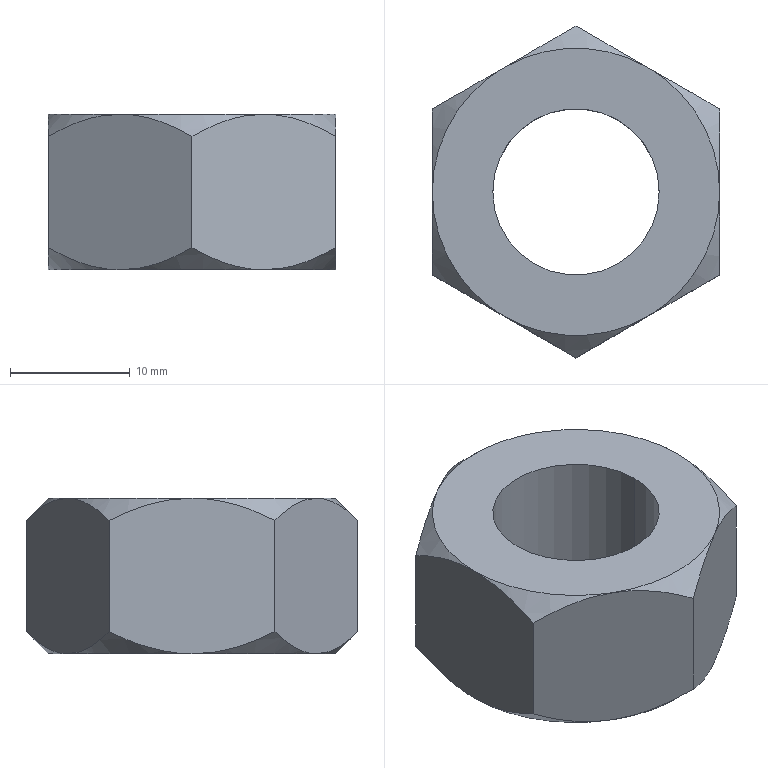Part | NX | 1 solid | 22 faces | box 24 x 27.713 x 13 mm | volume 4460 mm3 | cone 12 | plane 8 | cylinder 2 | commonest cylinder face diameters 13.9 x2
STEP:
#1=CARTESIAN_POINT('',(6.,-10.392,-6.5));
#2=VERTEX_POINT('',#1);
#3=CARTESIAN_POINT('',(12.,0.,-6.5));
#4=VERTEX_POINT('',#3);
#5=CARTESIAN_POINT('',(0.,0.,-6.5));
#6=DIRECTION('',(0.,0.,1.));
#7=DIRECTION('',(0.5,-0.866,0.));
#8=AXIS2_PLACEMENT_3D('',#5,#6,#7);
#9=CIRCLE('',#8,12.);
#10=EDGE_CURVE('',#2,#4,#9,.T.);
#11=ORIENTED_EDGE('',*,*,#10,.F.);
#12=CARTESIAN_POINT('',(-6.,-10.392,-6.5));
#13=VERTEX_POINT('',#12);
#14=CARTESIAN_POINT('',(0.,0.,-6.5));
#15=DIRECTION('',(0.,0.,1.));
#16=DIRECTION('',(-0.5,-0.866,0.));
#17=AXIS2_PLACEMENT_3D('',#14,#15,#16);
#18=CIRCLE('',#17,12.);
#19=EDGE_CURVE('',#13,#2,#18,.T.);
#20=ORIENTED_EDGE('',*,*,#19,.F.);
#21=CARTESIAN_POINT('',(-12.,0.,-6.5));
#22=VERTEX_POINT('',#21);
#23=CARTESIAN_POINT('',(0.,0.,-6.5));
#24=DIRECTION('',(0.,0.,1.));
#25=DIRECTION('',(-1.,0.,0.));
#26=AXIS2_PLACEMENT_3D('',#23,#24,#25);
#27=CIRCLE('',#26,12.);
#28=EDGE_CURVE('',#22,#13,#27,.T.);
#29=ORIENTED_EDGE('',*,*,#28,.F.);
#30=CARTESIAN_POINT('',(-6.,10.392,-6.5));
#31=VERTEX_POINT('',#30);
#32=CARTESIAN_POINT('',(0.,0.,-6.5));
#33=DIRECTION('',(0.,0.,1.));
#34=DIRECTION('',(-0.5,0.866,0.));
#35=AXIS2_PLACEMENT_3D('',#32,#33,#34);
#36=CIRCLE('',#35,12.);
#37=EDGE_CURVE('',#31,#22,#36,.T.);
#38=ORIENTED_EDGE('',*,*,#37,.F.);
#39=CARTESIAN_POINT('',(6.,10.392,-6.5));
#40=VERTEX_POINT('',#39);
#41=CARTESIAN_POINT('',(0.,0.,-6.5));
#42=DIRECTION('',(0.,0.,1.));
#43=DIRECTION('',(0.5,0.866,0.));
#44=AXIS2_PLACEMENT_3D('',#41,#42,#43);
#45=CIRCLE('',#44,12.);
#46=EDGE_CURVE('',#40,#31,#45,.T.);
#47=ORIENTED_EDGE('',*,*,#46,.F.);
#48=CARTESIAN_POINT('',(0.,0.,-6.5));
#49=DIRECTION('',(0.,0.,1.));
#50=DIRECTION('',(1.,0.,0.));
#51=AXIS2_PLACEMENT_3D('',#48,#49,#50);
#52=CIRCLE('',#51,12.);
#53=EDGE_CURVE('',#4,#40,#52,.T.);
#54=ORIENTED_EDGE('',*,*,#53,.F.);
#55=EDGE_LOOP('',(#11,#20,#29,#38,#47,#54));
#56=FACE_BOUND('',#55,.T.);
#57=CARTESIAN_POINT('',(-6.95,0.,-6.5));
#58=VERTEX_POINT('',#57);
#59=CARTESIAN_POINT('',(6.95,0.,-6.5));
#60=VERTEX_POINT('',#59);
#61=CARTESIAN_POINT('',(0.,0.,-6.5));
#62=DIRECTION('',(0.,0.,-1.));
#63=DIRECTION('',(1.,0.,0.));
#64=AXIS2_PLACEMENT_3D('',#61,#62,#63);
#65=CIRCLE('',#64,6.95);
#66=EDGE_CURVE('',#58,#60,#65,.T.);
#67=ORIENTED_EDGE('',*,*,#66,.F.);
#68=CARTESIAN_POINT('',(0.,0.,-6.5));
#69=DIRECTION('',(0.,0.,-1.));
#70=DIRECTION('',(1.,0.,0.));
#71=AXIS2_PLACEMENT_3D('',#68,#69,#70);
#72=CIRCLE('',#71,6.95);
#73=EDGE_CURVE('',#60,#58,#72,.T.);
#74=ORIENTED_EDGE('',*,*,#73,.F.);
#75=EDGE_LOOP('',(#67,#74));
#76=FACE_BOUND('',#75,.T.);
#77=CARTESIAN_POINT('',(0.,0.,-6.5));
#78=DIRECTION('',(0.,0.,1.));
#79=DIRECTION('',(1.,0.,0.));
#80=AXIS2_PLACEMENT_3D('',#77,#78,#79);
#81=PLANE('',#80);
#82=ADVANCED_FACE('',(#56,#76),#81,.F.);
#83=CARTESIAN_POINT('',(12.,-6.928,-4.644));
#84=VERTEX_POINT('',#83);
#85=CARTESIAN_POINT('',(6.,-10.392,-6.5));
#86=CARTESIAN_POINT('',(6.475,-10.118,-6.5));
#87=CARTESIAN_POINT('',(7.398,-9.585,-6.434));
#88=CARTESIAN_POINT('',(8.971,-8.677,-6.056));
#89=CARTESIAN_POINT('',(10.395,-7.855,-5.504));
#90=CARTESIAN_POINT('',(11.458,-7.241,-4.957));
#91=CARTESIAN_POINT('',(12.,-6.928,-4.644));
#92=B_SPLINE_CURVE_WITH_KNOTS('',3,(#85,#86,#87,#88,#89,#90,#91),.UNSPECIFIED.,.F.,.F.,(4,1,1,1,4),(0.,0.25,0.5,0.75,1.),.UNSPECIFIED.);
#93=EDGE_CURVE('',#2,#84,#92,.T.);
#94=ORIENTED_EDGE('',*,*,#93,.F.);
#95=ORIENTED_EDGE('',*,*,#10,.T.);
#96=CARTESIAN_POINT('',(12.,-6.928,-4.644));
#97=CARTESIAN_POINT('',(12.,-6.287,-4.964));
#98=CARTESIAN_POINT('',(12.,-5.009,-5.531));
#99=CARTESIAN_POINT('',(12.,-2.828,-6.249));
#100=CARTESIAN_POINT('',(12.,-1.102,-6.5));
#101=CARTESIAN_POINT('',(12.,0.,-6.5));
#102=B_SPLINE_CURVE_WITH_KNOTS('',3,(#96,#97,#98,#99,#100,#101),.UNSPECIFIED.,.F.,.F.,(4,1,1,4),(0.,0.25,0.5,1.),.UNSPECIFIED.);
#103=EDGE_CURVE('',#84,#4,#102,.T.);
#104=ORIENTED_EDGE('',*,*,#103,.F.);
#105=EDGE_LOOP('',(#94,#95,#104));
#106=FACE_BOUND('',#105,.T.);
#107=CARTESIAN_POINT('',(0.,0.,-5.572));
#108=DIRECTION('',(0.,0.,1.));
#109=DIRECTION('',(1.,0.,0.));
#110=AXIS2_PLACEMENT_3D('',#107,#108,#109);
#111=CONICAL_SURFACE('',#110,12.928,0.7854);
#112=ADVANCED_FACE('',(#106),#111,.T.);
#113=ORIENTED_EDGE('',*,*,#93,.T.);
#114=CARTESIAN_POINT('',(12.,-6.928,4.644));
#115=VERTEX_POINT('',#114);
#116=CARTESIAN_POINT('',(12.,-6.928,4.644));
#117=DIRECTION('',(0.,0.,-1.));
#118=VECTOR('',#117,1000.);
#119=LINE('',#116,#118);
#120=EDGE_CURVE('',#115,#84,#119,.T.);
#121=ORIENTED_EDGE('',*,*,#120,.F.);
#122=CARTESIAN_POINT('',(6.,-10.392,6.5));
#123=VERTEX_POINT('',#122);
#124=CARTESIAN_POINT('',(12.,-6.928,4.644));
#125=CARTESIAN_POINT('',(11.516,-7.207,4.923));
#126=CARTESIAN_POINT('',(10.816,-7.612,5.291));
#127=CARTESIAN_POINT('',(9.884,-8.15,5.695));
#128=CARTESIAN_POINT('',(9.281,-8.498,5.926));
#129=CARTESIAN_POINT('',(8.399,-9.007,6.198));
#130=CARTESIAN_POINT('',(7.335,-9.621,6.426));
#131=CARTESIAN_POINT('',(6.528,-10.088,6.5));
#132=CARTESIAN_POINT('',(6.,-10.392,6.5));
#133=B_SPLINE_CURVE_WITH_KNOTS('',3,(#124,#125,#126,#127,#128,#129,#130,#131,#132),.UNSPECIFIED.,.F.,.F.,(4,1,1,1,1,1,4),(0.,0.25,0.375,0.5,0.625,0.75,1.),.UNSPECIFIED.);
#134=EDGE_CURVE('',#123,#115,#133,.F.);
#135=ORIENTED_EDGE('',*,*,#134,.F.);
#136=CARTESIAN_POINT('',(0.,-13.856,4.644));
#137=VERTEX_POINT('',#136);
#138=CARTESIAN_POINT('',(6.,-10.392,6.5));
#139=CARTESIAN_POINT('',(5.525,-10.667,6.5));
#140=CARTESIAN_POINT('',(4.602,-11.2,6.434));
#141=CARTESIAN_POINT('',(3.029,-12.108,6.056));
#142=CARTESIAN_POINT('',(1.605,-12.93,5.504));
#143=CARTESIAN_POINT('',(0.5422,-13.543,4.957));
#144=CARTESIAN_POINT('',(0.,-13.856,4.644));
#145=B_SPLINE_CURVE_WITH_KNOTS('',3,(#138,#139,#140,#141,#142,#143,#144),.UNSPECIFIED.,.F.,.F.,(4,1,1,1,4),(0.,0.25,0.5,0.75,1.),.UNSPECIFIED.);
#146=EDGE_CURVE('',#123,#137,#145,.T.);
#147=ORIENTED_EDGE('',*,*,#146,.T.);
#148=CARTESIAN_POINT('',(0.,-13.856,-4.644));
#149=VERTEX_POINT('',#148);
#150=CARTESIAN_POINT('',(0.,-13.856,4.644));
#151=DIRECTION('',(0.,0.,-1.));
#152=VECTOR('',#151,1000.);
#153=LINE('',#150,#152);
#154=EDGE_CURVE('',#137,#149,#153,.T.);
#155=ORIENTED_EDGE('',*,*,#154,.T.);
#156=CARTESIAN_POINT('',(0.,-13.856,-4.644));
#157=CARTESIAN_POINT('',(0.2261,-13.726,-4.774));
#158=CARTESIAN_POINT('',(0.6703,-13.469,-5.019));
#159=CARTESIAN_POINT('',(1.31,-13.1,-5.34));
#160=CARTESIAN_POINT('',(1.929,-12.743,-5.618));
#161=CARTESIAN_POINT('',(2.532,-12.395,-5.855));
#162=CARTESIAN_POINT('',(3.124,-12.053,-6.055));
#163=CARTESIAN_POINT('',(3.707,-11.716,-6.217));
#164=CARTESIAN_POINT('',(4.285,-11.382,-6.344));
#165=CARTESIAN_POINT('',(4.859,-11.051,-6.434));
#166=CARTESIAN_POINT('',(5.43,-10.722,-6.488));
#167=CARTESIAN_POINT('',(5.81,-10.502,-6.5));
#168=CARTESIAN_POINT('',(6.,-10.392,-6.5));
#169=B_SPLINE_CURVE_WITH_KNOTS('',3,(#156,#157,#158,#159,#160,#161,#162,#163,#164,#165,#166,#167,#168),.UNSPECIFIED.,.F.,.F.,(4,1,1,1,1,1,1,1,1,1,4),(0.,0.1,0.2,0.3,0.4,0.5,0.6,0.7,0.8,0.9,1.),.UNSPECIFIED.);
#170=EDGE_CURVE('',#149,#2,#169,.T.);
#171=ORIENTED_EDGE('',*,*,#170,.T.);
#172=EDGE_LOOP('',(#113,#121,#135,#147,#155,#171));
#173=FACE_BOUND('',#172,.T.);
#174=CARTESIAN_POINT('',(0.,-13.856,-6.5));
#175=DIRECTION('',(0.5,-0.866,0.));
#176=DIRECTION('',(0.,0.,-1.));
#177=AXIS2_PLACEMENT_3D('',#174,#175,#176);
#178=PLANE('',#177);
#179=ADVANCED_FACE('',(#173),#178,.T.);
#180=CARTESIAN_POINT('',(-6.,-10.392,-6.5));
#181=CARTESIAN_POINT('',(-5.525,-10.666,-6.5));
#182=CARTESIAN_POINT('',(-4.602,-11.199,-6.434));
#183=CARTESIAN_POINT('',(-3.029,-12.108,-6.056));
#184=CARTESIAN_POINT('',(-1.605,-12.93,-5.504));
#185=CARTESIAN_POINT('',(-0.5422,-13.543,-4.957));
#186=CARTESIAN_POINT('',(0.,-13.856,-4.644));
#187=B_SPLINE_CURVE_WITH_KNOTS('',3,(#180,#181,#182,#183,#184,#185,#186),.UNSPECIFIED.,.F.,.F.,(4,1,1,1,4),(0.,0.25,0.5,0.75,1.),.UNSPECIFIED.);
#188=EDGE_CURVE('',#13,#149,#187,.T.);
#189=ORIENTED_EDGE('',*,*,#188,.F.);
#190=ORIENTED_EDGE('',*,*,#19,.T.);
#191=ORIENTED_EDGE('',*,*,#170,.F.);
#192=EDGE_LOOP('',(#189,#190,#191));
#193=FACE_BOUND('',#192,.T.);
#194=CARTESIAN_POINT('',(0.,0.,-5.572));
#195=DIRECTION('',(0.,0.,1.));
#196=DIRECTION('',(1.,0.,0.));
#197=AXIS2_PLACEMENT_3D('',#194,#195,#196);
#198=CONICAL_SURFACE('',#197,12.928,0.7854);
#199=ADVANCED_FACE('',(#193),#198,.T.);
#200=ORIENTED_EDGE('',*,*,#188,.T.);
#201=ORIENTED_EDGE('',*,*,#154,.F.);
#202=CARTESIAN_POINT('',(-6.,-10.392,6.5));
#203=VERTEX_POINT('',#202);
#204=CARTESIAN_POINT('',(0.,-13.856,4.644));
#205=CARTESIAN_POINT('',(-0.4837,-13.577,4.923));
#206=CARTESIAN_POINT('',(-1.184,-13.173,5.291));
#207=CARTESIAN_POINT('',(-2.116,-12.635,5.695));
#208=CARTESIAN_POINT('',(-2.719,-12.286,5.926));
#209=CARTESIAN_POINT('',(-3.601,-11.777,6.198));
#210=CARTESIAN_POINT('',(-4.665,-11.163,6.426));
#211=CARTESIAN_POINT('',(-5.472,-10.697,6.5));
#212=CARTESIAN_POINT('',(-6.,-10.392,6.5));
#213=B_SPLINE_CURVE_WITH_KNOTS('',3,(#204,#205,#206,#207,#208,#209,#210,#211,#212),.UNSPECIFIED.,.F.,.F.,(4,1,1,1,1,1,4),(0.,0.25,0.375,0.5,0.625,0.75,1.),.UNSPECIFIED.);
#214=EDGE_CURVE('',#203,#137,#213,.F.);
#215=ORIENTED_EDGE('',*,*,#214,.F.);
#216=CARTESIAN_POINT('',(-12.,-6.928,4.644));
#217=VERTEX_POINT('',#216);
#218=CARTESIAN_POINT('',(-6.,-10.392,6.5));
#219=CARTESIAN_POINT('',(-6.475,-10.118,6.5));
#220=CARTESIAN_POINT('',(-7.398,-9.585,6.434));
#221=CARTESIAN_POINT('',(-8.971,-8.677,6.056));
#222=CARTESIAN_POINT('',(-10.395,-7.855,5.504));
#223=CARTESIAN_POINT('',(-11.458,-7.241,4.957));
#224=CARTESIAN_POINT('',(-12.,-6.928,4.644));
#225=B_SPLINE_CURVE_WITH_KNOTS('',3,(#218,#219,#220,#221,#222,#223,#224),.UNSPECIFIED.,.F.,.F.,(4,1,1,1,4),(0.,0.25,0.5,0.75,1.),.UNSPECIFIED.);
#226=EDGE_CURVE('',#203,#217,#225,.T.);
#227=ORIENTED_EDGE('',*,*,#226,.T.);
#228=CARTESIAN_POINT('',(-12.,-6.928,-4.644));
#229=VERTEX_POINT('',#228);
#230=CARTESIAN_POINT('',(-12.,-6.928,4.644));
#231=DIRECTION('',(0.,0.,-1.));
#232=VECTOR('',#231,1000.);
#233=LINE('',#230,#232);
#234=EDGE_CURVE('',#217,#229,#233,.T.);
#235=ORIENTED_EDGE('',*,*,#234,.T.);
#236=CARTESIAN_POINT('',(-12.,-6.928,-4.644));
#237=CARTESIAN_POINT('',(-11.774,-7.059,-4.774));
#238=CARTESIAN_POINT('',(-11.33,-7.315,-5.019));
#239=CARTESIAN_POINT('',(-10.69,-7.684,-5.34));
#240=CARTESIAN_POINT('',(-10.071,-8.042,-5.618));
#241=CARTESIAN_POINT('',(-9.468,-8.39,-5.855));
#242=CARTESIAN_POINT('',(-8.876,-8.732,-6.055));
#243=CARTESIAN_POINT('',(-8.293,-9.069,-6.217));
#244=CARTESIAN_POINT('',(-7.715,-9.402,-6.344));
#245=CARTESIAN_POINT('',(-7.141,-9.733,-6.434));
#246=CARTESIAN_POINT('',(-6.57,-10.063,-6.488));
#247=CARTESIAN_POINT('',(-6.19,-10.283,-6.5));
#248=CARTESIAN_POINT('',(-6.,-10.392,-6.5));
#249=B_SPLINE_CURVE_WITH_KNOTS('',3,(#236,#237,#238,#239,#240,#241,#242,#243,#244,#245,#246,#247,#248),.UNSPECIFIED.,.F.,.F.,(4,1,1,1,1,1,1,1,1,1,4),(0.,0.1,0.2,0.3,0.4,0.5,0.6,0.7,0.8,0.9,1.),.UNSPECIFIED.);
#250=EDGE_CURVE('',#229,#13,#249,.T.);
#251=ORIENTED_EDGE('',*,*,#250,.T.);
#252=EDGE_LOOP('',(#200,#201,#215,#227,#235,#251));
#253=FACE_BOUND('',#252,.T.);
#254=CARTESIAN_POINT('',(-12.,-6.928,-6.5));
#255=DIRECTION('',(-0.5,-0.866,0.));
#256=DIRECTION('',(-0.866,0.5,0.));
#257=AXIS2_PLACEMENT_3D('',#254,#255,#256);
#258=PLANE('',#257);
#259=ADVANCED_FACE('',(#253),#258,.T.);
#260=CARTESIAN_POINT('',(-12.,0.,-6.5));
#261=CARTESIAN_POINT('',(-12.,-0.5482,-6.5));
#262=CARTESIAN_POINT('',(-12.,-1.614,-6.434));
#263=CARTESIAN_POINT('',(-12.,-3.43,-6.056));
#264=CARTESIAN_POINT('',(-12.,-5.075,-5.504));
#265=CARTESIAN_POINT('',(-12.,-6.302,-4.957));
#266=CARTESIAN_POINT('',(-12.,-6.928,-4.644));
#267=B_SPLINE_CURVE_WITH_KNOTS('',3,(#260,#261,#262,#263,#264,#265,#266),.UNSPECIFIED.,.F.,.F.,(4,1,1,1,4),(0.,0.25,0.5,0.75,1.),.UNSPECIFIED.);
#268=EDGE_CURVE('',#22,#229,#267,.T.);
#269=ORIENTED_EDGE('',*,*,#268,.F.);
#270=ORIENTED_EDGE('',*,*,#28,.T.);
#271=ORIENTED_EDGE('',*,*,#250,.F.);
#272=EDGE_LOOP('',(#269,#270,#271));
#273=FACE_BOUND('',#272,.T.);
#274=CARTESIAN_POINT('',(0.,0.,-5.572));
#275=DIRECTION('',(0.,0.,1.));
#276=DIRECTION('',(1.,0.,0.));
#277=AXIS2_PLACEMENT_3D('',#274,#275,#276);
#278=CONICAL_SURFACE('',#277,12.928,0.7854);
#279=ADVANCED_FACE('',(#273),#278,.T.);
#280=ORIENTED_EDGE('',*,*,#268,.T.);
#281=ORIENTED_EDGE('',*,*,#234,.F.);
#282=CARTESIAN_POINT('',(-12.,0.,6.5));
#283=VERTEX_POINT('',#282);
#284=CARTESIAN_POINT('',(-12.,-6.928,4.644));
#285=CARTESIAN_POINT('',(-12.,-6.364,4.926));
#286=CARTESIAN_POINT('',(-12.,-5.545,5.298));
#287=CARTESIAN_POINT('',(-12.,-4.461,5.704));
#288=CARTESIAN_POINT('',(-12.,-3.75,5.937));
#289=CARTESIAN_POINT('',(-12.,-2.746,6.203));
#290=CARTESIAN_POINT('',(-12.,-1.527,6.428));
#291=CARTESIAN_POINT('',(-12.,-0.6038,6.5));
#292=CARTESIAN_POINT('',(-12.,0.,6.5));
#293=B_SPLINE_CURVE_WITH_KNOTS('',3,(#284,#285,#286,#287,#288,#289,#290,#291,#292),.UNSPECIFIED.,.F.,.F.,(4,1,1,1,1,1,4),(0.,0.25,0.375,0.5,0.625,0.75,1.),.UNSPECIFIED.);
#294=EDGE_CURVE('',#283,#217,#293,.F.);
#295=ORIENTED_EDGE('',*,*,#294,.F.);
#296=CARTESIAN_POINT('',(-12.,6.928,4.644));
#297=VERTEX_POINT('',#296);
#298=CARTESIAN_POINT('',(-12.,0.,6.5));
#299=CARTESIAN_POINT('',(-12.,0.5482,6.5));
#300=CARTESIAN_POINT('',(-12.,1.614,6.434));
#301=CARTESIAN_POINT('',(-12.,3.43,6.057));
#302=CARTESIAN_POINT('',(-12.,5.075,5.504));
#303=CARTESIAN_POINT('',(-12.,6.302,4.957));
#304=CARTESIAN_POINT('',(-12.,6.928,4.644));
#305=B_SPLINE_CURVE_WITH_KNOTS('',3,(#298,#299,#300,#301,#302,#303,#304),.UNSPECIFIED.,.F.,.F.,(4,1,1,1,4),(0.,0.25,0.5,0.75,1.),.UNSPECIFIED.);
#306=EDGE_CURVE('',#283,#297,#305,.T.);
#307=ORIENTED_EDGE('',*,*,#306,.T.);
#308=CARTESIAN_POINT('',(-12.,6.928,-4.644));
#309=VERTEX_POINT('',#308);
#310=CARTESIAN_POINT('',(-12.,6.928,4.644));
#311=DIRECTION('',(0.,0.,-1.));
#312=VECTOR('',#311,1000.);
#313=LINE('',#310,#312);
#314=EDGE_CURVE('',#297,#309,#313,.T.);
#315=ORIENTED_EDGE('',*,*,#314,.T.);
#316=CARTESIAN_POINT('',(-12.,6.928,-4.644));
#317=CARTESIAN_POINT('',(-12.,6.287,-4.964));
#318=CARTESIAN_POINT('',(-12.,5.009,-5.531));
#319=CARTESIAN_POINT('',(-12.,2.828,-6.249));
#320=CARTESIAN_POINT('',(-12.,1.102,-6.5));
#321=CARTESIAN_POINT('',(-12.,0.,-6.5));
#322=B_SPLINE_CURVE_WITH_KNOTS('',3,(#316,#317,#318,#319,#320,#321),.UNSPECIFIED.,.F.,.F.,(4,1,1,4),(0.,0.25,0.5,1.),.UNSPECIFIED.);
#323=EDGE_CURVE('',#309,#22,#322,.T.);
#324=ORIENTED_EDGE('',*,*,#323,.T.);
#325=EDGE_LOOP('',(#280,#281,#295,#307,#315,#324));
#326=FACE_BOUND('',#325,.T.);
#327=CARTESIAN_POINT('',(-12.,6.928,-6.5));
#328=DIRECTION('',(-1.,0.,0.));
#329=DIRECTION('',(0.,0.,1.));
#330=AXIS2_PLACEMENT_3D('',#327,#328,#329);
#331=PLANE('',#330);
#332=ADVANCED_FACE('',(#326),#331,.T.);
#333=CARTESIAN_POINT('',(-6.,10.392,-6.5));
#334=CARTESIAN_POINT('',(-6.475,10.118,-6.5));
#335=CARTESIAN_POINT('',(-7.398,9.585,-6.434));
#336=CARTESIAN_POINT('',(-8.971,8.677,-6.056));
#337=CARTESIAN_POINT('',(-10.395,7.855,-5.504));
#338=CARTESIAN_POINT('',(-11.458,7.241,-4.957));
#339=CARTESIAN_POINT('',(-12.,6.928,-4.644));
#340=B_SPLINE_CURVE_WITH_KNOTS('',3,(#333,#334,#335,#336,#337,#338,#339),.UNSPECIFIED.,.F.,.F.,(4,1,1,1,4),(0.,0.25,0.5,0.75,1.),.UNSPECIFIED.);
#341=EDGE_CURVE('',#31,#309,#340,.T.);
#342=ORIENTED_EDGE('',*,*,#341,.F.);
#343=ORIENTED_EDGE('',*,*,#37,.T.);
#344=ORIENTED_EDGE('',*,*,#323,.F.);
#345=EDGE_LOOP('',(#342,#343,#344));
#346=FACE_BOUND('',#345,.T.);
#347=CARTESIAN_POINT('',(0.,0.,-5.572));
#348=DIRECTION('',(0.,0.,1.));
#349=DIRECTION('',(1.,0.,0.));
#350=AXIS2_PLACEMENT_3D('',#347,#348,#349);
#351=CONICAL_SURFACE('',#350,12.928,0.7854);
#352=ADVANCED_FACE('',(#346),#351,.T.);
#353=ORIENTED_EDGE('',*,*,#341,.T.);
#354=ORIENTED_EDGE('',*,*,#314,.F.);
#355=CARTESIAN_POINT('',(-6.,10.392,6.5));
#356=VERTEX_POINT('',#355);
#357=CARTESIAN_POINT('',(-12.,6.928,4.644));
#358=CARTESIAN_POINT('',(-11.516,7.207,4.923));
#359=CARTESIAN_POINT('',(-10.816,7.612,5.291));
#360=CARTESIAN_POINT('',(-9.884,8.15,5.695));
#361=CARTESIAN_POINT('',(-9.281,8.498,5.926));
#362=CARTESIAN_POINT('',(-8.399,9.007,6.198));
#363=CARTESIAN_POINT('',(-7.335,9.621,6.426));
#364=CARTESIAN_POINT('',(-6.528,10.088,6.5));
#365=CARTESIAN_POINT('',(-6.,10.392,6.5));
#366=B_SPLINE_CURVE_WITH_KNOTS('',3,(#357,#358,#359,#360,#361,#362,#363,#364,#365),.UNSPECIFIED.,.F.,.F.,(4,1,1,1,1,1,4),(0.,0.25,0.375,0.5,0.625,0.75,1.),.UNSPECIFIED.);
#367=EDGE_CURVE('',#356,#297,#366,.F.);
#368=ORIENTED_EDGE('',*,*,#367,.F.);
#369=CARTESIAN_POINT('',(0.,13.856,4.644));
#370=VERTEX_POINT('',#369);
#371=CARTESIAN_POINT('',(-6.,10.392,6.5));
#372=CARTESIAN_POINT('',(-5.525,10.667,6.5));
#373=CARTESIAN_POINT('',(-4.602,11.2,6.434));
#374=CARTESIAN_POINT('',(-3.029,12.108,6.056));
#375=CARTESIAN_POINT('',(-1.605,12.93,5.504));
#376=CARTESIAN_POINT('',(-0.5422,13.543,4.957));
#377=CARTESIAN_POINT('',(0.,13.856,4.644));
#378=B_SPLINE_CURVE_WITH_KNOTS('',3,(#371,#372,#373,#374,#375,#376,#377),.UNSPECIFIED.,.F.,.F.,(4,1,1,1,4),(0.,0.25,0.5,0.75,1.),.UNSPECIFIED.);
#379=EDGE_CURVE('',#356,#370,#378,.T.);
#380=ORIENTED_EDGE('',*,*,#379,.T.);
#381=CARTESIAN_POINT('',(0.,13.856,-4.644));
#382=VERTEX_POINT('',#381);
#383=CARTESIAN_POINT('',(0.,13.856,4.644));
#384=DIRECTION('',(0.,0.,-1.));
#385=VECTOR('',#384,1000.);
#386=LINE('',#383,#385);
#387=EDGE_CURVE('',#370,#382,#386,.T.);
#388=ORIENTED_EDGE('',*,*,#387,.T.);
#389=CARTESIAN_POINT('',(0.,13.856,-4.644));
#390=CARTESIAN_POINT('',(-0.2261,13.726,-4.774));
#391=CARTESIAN_POINT('',(-0.6703,13.469,-5.019));
#392=CARTESIAN_POINT('',(-1.31,13.1,-5.34));
#393=CARTESIAN_POINT('',(-1.929,12.743,-5.618));
#394=CARTESIAN_POINT('',(-2.532,12.395,-5.855));
#395=CARTESIAN_POINT('',(-3.124,12.053,-6.055));
#396=CARTESIAN_POINT('',(-3.707,11.716,-6.217));
#397=CARTESIAN_POINT('',(-4.285,11.382,-6.344));
#398=CARTESIAN_POINT('',(-4.859,11.051,-6.434));
#399=CARTESIAN_POINT('',(-5.43,10.722,-6.488));
#400=CARTESIAN_POINT('',(-5.81,10.502,-6.5));
#401=CARTESIAN_POINT('',(-6.,10.392,-6.5));
#402=B_SPLINE_CURVE_WITH_KNOTS('',3,(#389,#390,#391,#392,#393,#394,#395,#396,#397,#398,#399,#400,#401),.UNSPECIFIED.,.F.,.F.,(4,1,1,1,1,1,1,1,1,1,4),(0.,0.1,0.2,0.3,0.4,0.5,0.6,0.7,0.8,0.9,1.),.UNSPECIFIED.);
#403=EDGE_CURVE('',#382,#31,#402,.T.);
#404=ORIENTED_EDGE('',*,*,#403,.T.);
#405=EDGE_LOOP('',(#353,#354,#368,#380,#388,#404));
#406=FACE_BOUND('',#405,.T.);
#407=CARTESIAN_POINT('',(0.,13.856,-6.5));
#408=DIRECTION('',(-0.5,0.866,0.));
#409=DIRECTION('',(0.,0.,1.));
#410=AXIS2_PLACEMENT_3D('',#407,#408,#409);
#411=PLANE('',#410);
#412=ADVANCED_FACE('',(#406),#411,.T.);
#413=CARTESIAN_POINT('',(6.,10.392,-6.5));
#414=CARTESIAN_POINT('',(5.525,10.666,-6.5));
#415=CARTESIAN_POINT('',(4.602,11.199,-6.434));
#416=CARTESIAN_POINT('',(3.029,12.108,-6.056));
#417=CARTESIAN_POINT('',(1.605,12.93,-5.504));
#418=CARTESIAN_POINT('',(0.5422,13.543,-4.957));
#419=CARTESIAN_POINT('',(0.,13.856,-4.644));
#420=B_SPLINE_CURVE_WITH_KNOTS('',3,(#413,#414,#415,#416,#417,#418,#419),.UNSPECIFIED.,.F.,.F.,(4,1,1,1,4),(0.,0.25,0.5,0.75,1.),.UNSPECIFIED.);
#421=EDGE_CURVE('',#40,#382,#420,.T.);
#422=ORIENTED_EDGE('',*,*,#421,.F.);
#423=ORIENTED_EDGE('',*,*,#46,.T.);
#424=ORIENTED_EDGE('',*,*,#403,.F.);
#425=EDGE_LOOP('',(#422,#423,#424));
#426=FACE_BOUND('',#425,.T.);
#427=CARTESIAN_POINT('',(0.,0.,-5.572));
#428=DIRECTION('',(0.,0.,1.));
#429=DIRECTION('',(1.,0.,0.));
#430=AXIS2_PLACEMENT_3D('',#427,#428,#429);
#431=CONICAL_SURFACE('',#430,12.928,0.7854);
#432=ADVANCED_FACE('',(#426),#431,.T.);
#433=ORIENTED_EDGE('',*,*,#421,.T.);
#434=ORIENTED_EDGE('',*,*,#387,.F.);
#435=CARTESIAN_POINT('',(6.,10.392,6.5));
#436=VERTEX_POINT('',#435);
#437=CARTESIAN_POINT('',(0.,13.856,4.644));
#438=CARTESIAN_POINT('',(0.4837,13.577,4.923));
#439=CARTESIAN_POINT('',(1.184,13.173,5.291));
#440=CARTESIAN_POINT('',(2.116,12.635,5.695));
#441=CARTESIAN_POINT('',(2.719,12.286,5.926));
#442=CARTESIAN_POINT('',(3.601,11.777,6.198));
#443=CARTESIAN_POINT('',(4.665,11.163,6.426));
#444=CARTESIAN_POINT('',(5.472,10.697,6.5));
#445=CARTESIAN_POINT('',(6.,10.392,6.5));
#446=B_SPLINE_CURVE_WITH_KNOTS('',3,(#437,#438,#439,#440,#441,#442,#443,#444,#445),.UNSPECIFIED.,.F.,.F.,(4,1,1,1,1,1,4),(0.,0.25,0.375,0.5,0.625,0.75,1.),.UNSPECIFIED.);
#447=EDGE_CURVE('',#436,#370,#446,.F.);
#448=ORIENTED_EDGE('',*,*,#447,.F.);
#449=CARTESIAN_POINT('',(12.,6.928,4.644));
#450=VERTEX_POINT('',#449);
#451=CARTESIAN_POINT('',(6.,10.392,6.5));
#452=CARTESIAN_POINT('',(6.475,10.118,6.5));
#453=CARTESIAN_POINT('',(7.398,9.585,6.434));
#454=CARTESIAN_POINT('',(8.971,8.677,6.056));
#455=CARTESIAN_POINT('',(10.395,7.855,5.504));
#456=CARTESIAN_POINT('',(11.458,7.241,4.957));
#457=CARTESIAN_POINT('',(12.,6.928,4.644));
#458=B_SPLINE_CURVE_WITH_KNOTS('',3,(#451,#452,#453,#454,#455,#456,#457),.UNSPECIFIED.,.F.,.F.,(4,1,1,1,4),(0.,0.25,0.5,0.75,1.),.UNSPECIFIED.);
#459=EDGE_CURVE('',#436,#450,#458,.T.);
#460=ORIENTED_EDGE('',*,*,#459,.T.);
#461=CARTESIAN_POINT('',(12.,6.928,-4.644));
#462=VERTEX_POINT('',#461);
#463=CARTESIAN_POINT('',(12.,6.928,4.644));
#464=DIRECTION('',(0.,0.,-1.));
#465=VECTOR('',#464,1000.);
#466=LINE('',#463,#465);
#467=EDGE_CURVE('',#450,#462,#466,.T.);
#468=ORIENTED_EDGE('',*,*,#467,.T.);
#469=CARTESIAN_POINT('',(12.,6.928,-4.644));
#470=CARTESIAN_POINT('',(11.774,7.059,-4.774));
#471=CARTESIAN_POINT('',(11.33,7.315,-5.019));
#472=CARTESIAN_POINT('',(10.69,7.684,-5.34));
#473=CARTESIAN_POINT('',(10.071,8.042,-5.618));
#474=CARTESIAN_POINT('',(9.468,8.39,-5.855));
#475=CARTESIAN_POINT('',(8.876,8.732,-6.055));
#476=CARTESIAN_POINT('',(8.293,9.069,-6.217));
#477=CARTESIAN_POINT('',(7.715,9.402,-6.344));
#478=CARTESIAN_POINT('',(7.141,9.733,-6.434));
#479=CARTESIAN_POINT('',(6.57,10.063,-6.488));
#480=CARTESIAN_POINT('',(6.19,10.283,-6.5));
#481=CARTESIAN_POINT('',(6.,10.392,-6.5));
#482=B_SPLINE_CURVE_WITH_KNOTS('',3,(#469,#470,#471,#472,#473,#474,#475,#476,#477,#478,#479,#480,#481),.UNSPECIFIED.,.F.,.F.,(4,1,1,1,1,1,1,1,1,1,4),(0.,0.1,0.2,0.3,0.4,0.5,0.6,0.7,0.8,0.9,1.),.UNSPECIFIED.);
#483=EDGE_CURVE('',#462,#40,#482,.T.);
#484=ORIENTED_EDGE('',*,*,#483,.T.);
#485=EDGE_LOOP('',(#433,#434,#448,#460,#468,#484));
#486=FACE_BOUND('',#485,.T.);
#487=CARTESIAN_POINT('',(12.,6.928,-6.5));
#488=DIRECTION('',(0.5,0.866,0.));
#489=DIRECTION('',(0.,0.,-1.));
#490=AXIS2_PLACEMENT_3D('',#487,#488,#489);
#491=PLANE('',#490);
#492=ADVANCED_FACE('',(#486),#491,.T.);
#493=CARTESIAN_POINT('',(12.,0.,-6.5));
#494=CARTESIAN_POINT('',(12.,0.5482,-6.5));
#495=CARTESIAN_POINT('',(12.,1.614,-6.434));
#496=CARTESIAN_POINT('',(12.,3.43,-6.056));
#497=CARTESIAN_POINT('',(12.,5.075,-5.504));
#498=CARTESIAN_POINT('',(12.,6.302,-4.957));
#499=CARTESIAN_POINT('',(12.,6.928,-4.644));
#500=B_SPLINE_CURVE_WITH_KNOTS('',3,(#493,#494,#495,#496,#497,#498,#499),.UNSPECIFIED.,.F.,.F.,(4,1,1,1,4),(0.,0.25,0.5,0.75,1.),.UNSPECIFIED.);
#501=EDGE_CURVE('',#4,#462,#500,.T.);
#502=ORIENTED_EDGE('',*,*,#501,.F.);
#503=ORIENTED_EDGE('',*,*,#53,.T.);
#504=ORIENTED_EDGE('',*,*,#483,.F.);
#505=EDGE_LOOP('',(#502,#503,#504));
#506=FACE_BOUND('',#505,.T.);
#507=CARTESIAN_POINT('',(0.,0.,-5.572));
#508=DIRECTION('',(0.,0.,1.));
#509=DIRECTION('',(1.,0.,0.));
#510=AXIS2_PLACEMENT_3D('',#507,#508,#509);
#511=CONICAL_SURFACE('',#510,12.928,0.7854);
#512=ADVANCED_FACE('',(#506),#511,.T.);
#513=ORIENTED_EDGE('',*,*,#103,.T.);
#514=ORIENTED_EDGE('',*,*,#501,.T.);
#515=ORIENTED_EDGE('',*,*,#467,.F.);
#516=CARTESIAN_POINT('',(12.,0.,6.5));
#517=VERTEX_POINT('',#516);
#518=CARTESIAN_POINT('',(12.,6.928,4.644));
#519=CARTESIAN_POINT('',(12.,6.364,4.926));
#520=CARTESIAN_POINT('',(12.,5.545,5.298));
#521=CARTESIAN_POINT('',(12.,4.461,5.704));
#522=CARTESIAN_POINT('',(12.,3.75,5.937));
#523=CARTESIAN_POINT('',(12.,2.746,6.203));
#524=CARTESIAN_POINT('',(12.,1.527,6.428));
#525=CARTESIAN_POINT('',(12.,0.6038,6.5));
#526=CARTESIAN_POINT('',(12.,0.,6.5));
#527=B_SPLINE_CURVE_WITH_KNOTS('',3,(#518,#519,#520,#521,#522,#523,#524,#525,#526),.UNSPECIFIED.,.F.,.F.,(4,1,1,1,1,1,4),(0.,0.25,0.375,0.5,0.625,0.75,1.),.UNSPECIFIED.);
#528=EDGE_CURVE('',#517,#450,#527,.F.);
#529=ORIENTED_EDGE('',*,*,#528,.F.);
#530=CARTESIAN_POINT('',(12.,0.,6.5));
#531=CARTESIAN_POINT('',(12.,-0.5482,6.5));
#532=CARTESIAN_POINT('',(12.,-1.614,6.434));
#533=CARTESIAN_POINT('',(12.,-3.43,6.057));
#534=CARTESIAN_POINT('',(12.,-5.075,5.504));
#535=CARTESIAN_POINT('',(12.,-6.302,4.957));
#536=CARTESIAN_POINT('',(12.,-6.928,4.644));
#537=B_SPLINE_CURVE_WITH_KNOTS('',3,(#530,#531,#532,#533,#534,#535,#536),.UNSPECIFIED.,.F.,.F.,(4,1,1,1,4),(0.,0.25,0.5,0.75,1.),.UNSPECIFIED.);
#538=EDGE_CURVE('',#517,#115,#537,.T.);
#539=ORIENTED_EDGE('',*,*,#538,.T.);
#540=ORIENTED_EDGE('',*,*,#120,.T.);
#541=EDGE_LOOP('',(#513,#514,#515,#529,#539,#540));
#542=FACE_BOUND('',#541,.T.);
#543=CARTESIAN_POINT('',(12.,-6.928,-6.5));
#544=DIRECTION('',(1.,0.,0.));
#545=DIRECTION('',(0.,1.,0.));
#546=AXIS2_PLACEMENT_3D('',#543,#544,#545);
#547=PLANE('',#546);
#548=ADVANCED_FACE('',(#542),#547,.T.);
#549=ORIENTED_EDGE('',*,*,#538,.F.);
#550=CARTESIAN_POINT('',(0.,0.,6.5));
#551=DIRECTION('',(0.,0.,-1.));
#552=DIRECTION('',(1.,0.,0.));
#553=AXIS2_PLACEMENT_3D('',#550,#551,#552);
#554=CIRCLE('',#553,12.);
#555=EDGE_CURVE('',#517,#123,#554,.T.);
#556=ORIENTED_EDGE('',*,*,#555,.T.);
#557=ORIENTED_EDGE('',*,*,#134,.T.);
#558=EDGE_LOOP('',(#549,#556,#557));
#559=FACE_BOUND('',#558,.T.);
#560=CARTESIAN_POINT('',(0.,0.,5.572));
#561=DIRECTION('',(0.,0.,-1.));
#562=DIRECTION('',(-1.,0.,0.));
#563=AXIS2_PLACEMENT_3D('',#560,#561,#562);
#564=CONICAL_SURFACE('',#563,12.928,0.7854);
#565=ADVANCED_FACE('',(#559),#564,.T.);
#566=ORIENTED_EDGE('',*,*,#555,.F.);
#567=CARTESIAN_POINT('',(0.,0.,6.5));
#568=DIRECTION('',(0.,0.,-1.));
#569=DIRECTION('',(0.5,0.866,0.));
#570=AXIS2_PLACEMENT_3D('',#567,#568,#569);
#571=CIRCLE('',#570,12.);
#572=EDGE_CURVE('',#436,#517,#571,.T.);
#573=ORIENTED_EDGE('',*,*,#572,.F.);
#574=CARTESIAN_POINT('',(0.,0.,6.5));
#575=DIRECTION('',(0.,0.,-1.));
#576=DIRECTION('',(-0.5,0.866,0.));
#577=AXIS2_PLACEMENT_3D('',#574,#575,#576);
#578=CIRCLE('',#577,12.);
#579=EDGE_CURVE('',#356,#436,#578,.T.);
#580=ORIENTED_EDGE('',*,*,#579,.F.);
#581=CARTESIAN_POINT('',(0.,0.,6.5));
#582=DIRECTION('',(0.,0.,-1.));
#583=DIRECTION('',(-1.,0.,0.));
#584=AXIS2_PLACEMENT_3D('',#581,#582,#583);
#585=CIRCLE('',#584,12.);
#586=EDGE_CURVE('',#283,#356,#585,.T.);
#587=ORIENTED_EDGE('',*,*,#586,.F.);
#588=CARTESIAN_POINT('',(0.,0.,6.5));
#589=DIRECTION('',(0.,0.,-1.));
#590=DIRECTION('',(-0.5,-0.866,0.));
#591=AXIS2_PLACEMENT_3D('',#588,#589,#590);
#592=CIRCLE('',#591,12.);
#593=EDGE_CURVE('',#203,#283,#592,.T.);
#594=ORIENTED_EDGE('',*,*,#593,.F.);
#595=CARTESIAN_POINT('',(0.,0.,6.5));
#596=DIRECTION('',(0.,0.,-1.));
#597=DIRECTION('',(0.5,-0.866,0.));
#598=AXIS2_PLACEMENT_3D('',#595,#596,#597);
#599=CIRCLE('',#598,12.);
#600=EDGE_CURVE('',#123,#203,#599,.T.);
#601=ORIENTED_EDGE('',*,*,#600,.F.);
#602=EDGE_LOOP('',(#566,#573,#580,#587,#594,#601));
#603=FACE_BOUND('',#602,.T.);
#604=CARTESIAN_POINT('',(6.95,0.,6.5));
#605=VERTEX_POINT('',#604);
#606=CARTESIAN_POINT('',(-6.95,0.,6.5));
#607=VERTEX_POINT('',#606);
#608=CARTESIAN_POINT('',(0.,0.,6.5));
#609=DIRECTION('',(0.,0.,1.));
#610=DIRECTION('',(-1.,0.,0.));
#611=AXIS2_PLACEMENT_3D('',#608,#609,#610);
#612=CIRCLE('',#611,6.95);
#613=EDGE_CURVE('',#605,#607,#612,.T.);
#614=ORIENTED_EDGE('',*,*,#613,.F.);
#615=CARTESIAN_POINT('',(0.,0.,6.5));
#616=DIRECTION('',(0.,0.,1.));
#617=DIRECTION('',(-1.,0.,0.));
#618=AXIS2_PLACEMENT_3D('',#615,#616,#617);
#619=CIRCLE('',#618,6.95);
#620=EDGE_CURVE('',#607,#605,#619,.T.);
#621=ORIENTED_EDGE('',*,*,#620,.F.);
#622=EDGE_LOOP('',(#614,#621));
#623=FACE_BOUND('',#622,.T.);
#624=CARTESIAN_POINT('',(0.,0.,6.5));
#625=DIRECTION('',(0.,0.,1.));
#626=DIRECTION('',(1.,0.,0.));
#627=AXIS2_PLACEMENT_3D('',#624,#625,#626);
#628=PLANE('',#627);
#629=ADVANCED_FACE('',(#603,#623),#628,.T.);
#630=ORIENTED_EDGE('',*,*,#146,.F.);
#631=ORIENTED_EDGE('',*,*,#600,.T.);
#632=ORIENTED_EDGE('',*,*,#214,.T.);
#633=EDGE_LOOP('',(#630,#631,#632));
#634=FACE_BOUND('',#633,.T.);
#635=CARTESIAN_POINT('',(0.,0.,5.572));
#636=DIRECTION('',(0.,0.,-1.));
#637=DIRECTION('',(-1.,0.,0.));
#638=AXIS2_PLACEMENT_3D('',#635,#636,#637);
#639=CONICAL_SURFACE('',#638,12.928,0.7854);
#640=ADVANCED_FACE('',(#634),#639,.T.);
#641=ORIENTED_EDGE('',*,*,#226,.F.);
#642=ORIENTED_EDGE('',*,*,#593,.T.);
#643=ORIENTED_EDGE('',*,*,#294,.T.);
#644=EDGE_LOOP('',(#641,#642,#643));
#645=FACE_BOUND('',#644,.T.);
#646=CARTESIAN_POINT('',(0.,0.,5.572));
#647=DIRECTION('',(0.,0.,-1.));
#648=DIRECTION('',(-1.,0.,0.));
#649=AXIS2_PLACEMENT_3D('',#646,#647,#648);
#650=CONICAL_SURFACE('',#649,12.928,0.7854);
#651=ADVANCED_FACE('',(#645),#650,.T.);
#652=ORIENTED_EDGE('',*,*,#306,.F.);
#653=ORIENTED_EDGE('',*,*,#586,.T.);
#654=ORIENTED_EDGE('',*,*,#367,.T.);
#655=EDGE_LOOP('',(#652,#653,#654));
#656=FACE_BOUND('',#655,.T.);
#657=CARTESIAN_POINT('',(0.,0.,5.572));
#658=DIRECTION('',(0.,0.,-1.));
#659=DIRECTION('',(-1.,0.,0.));
#660=AXIS2_PLACEMENT_3D('',#657,#658,#659);
#661=CONICAL_SURFACE('',#660,12.928,0.7854);
#662=ADVANCED_FACE('',(#656),#661,.T.);
#663=ORIENTED_EDGE('',*,*,#379,.F.);
#664=ORIENTED_EDGE('',*,*,#579,.T.);
#665=ORIENTED_EDGE('',*,*,#447,.T.);
#666=EDGE_LOOP('',(#663,#664,#665));
#667=FACE_BOUND('',#666,.T.);
#668=CARTESIAN_POINT('',(0.,0.,5.572));
#669=DIRECTION('',(0.,0.,-1.));
#670=DIRECTION('',(-1.,0.,0.));
#671=AXIS2_PLACEMENT_3D('',#668,#669,#670);
#672=CONICAL_SURFACE('',#671,12.928,0.7854);
#673=ADVANCED_FACE('',(#667),#672,.T.);
#674=ORIENTED_EDGE('',*,*,#459,.F.);
#675=ORIENTED_EDGE('',*,*,#572,.T.);
#676=ORIENTED_EDGE('',*,*,#528,.T.);
#677=EDGE_LOOP('',(#674,#675,#676));
#678=FACE_BOUND('',#677,.T.);
#679=CARTESIAN_POINT('',(0.,0.,5.572));
#680=DIRECTION('',(0.,0.,-1.));
#681=DIRECTION('',(-1.,0.,0.));
#682=AXIS2_PLACEMENT_3D('',#679,#680,#681);
#683=CONICAL_SURFACE('',#682,12.928,0.7854);
#684=ADVANCED_FACE('',(#678),#683,.T.);
#685=ORIENTED_EDGE('',*,*,#613,.T.);
#686=CARTESIAN_POINT('',(-6.95,0.,6.5));
#687=DIRECTION('',(0.,0.,-1.));
#688=VECTOR('',#687,1000.);
#689=LINE('',#686,#688);
#690=EDGE_CURVE('',#58,#607,#689,.F.);
#691=ORIENTED_EDGE('',*,*,#690,.F.);
#692=ORIENTED_EDGE('',*,*,#66,.T.);
#693=CARTESIAN_POINT('',(6.95,0.,6.5));
#694=DIRECTION('',(0.,0.,-1.));
#695=VECTOR('',#694,1000.);
#696=LINE('',#693,#695);
#697=EDGE_CURVE('',#60,#605,#696,.F.);
#698=ORIENTED_EDGE('',*,*,#697,.T.);
#699=EDGE_LOOP('',(#685,#691,#692,#698));
#700=FACE_BOUND('',#699,.T.);
#701=CARTESIAN_POINT('',(0.,0.,6.5));
#702=DIRECTION('',(0.,0.,-1.));
#703=DIRECTION('',(-1.,0.,0.));
#704=AXIS2_PLACEMENT_3D('',#701,#702,#703);
#705=CYLINDRICAL_SURFACE('',#704,6.95);
#706=ADVANCED_FACE('',(#700),#705,.F.);
#707=ORIENTED_EDGE('',*,*,#690,.T.);
#708=ORIENTED_EDGE('',*,*,#620,.T.);
#709=ORIENTED_EDGE('',*,*,#697,.F.);
#710=ORIENTED_EDGE('',*,*,#73,.T.);
#711=EDGE_LOOP('',(#707,#708,#709,#710));
#712=FACE_BOUND('',#711,.T.);
#713=CARTESIAN_POINT('',(0.,0.,6.5));
#714=DIRECTION('',(0.,0.,-1.));
#715=DIRECTION('',(-1.,0.,0.));
#716=AXIS2_PLACEMENT_3D('',#713,#714,#715);
#717=CYLINDRICAL_SURFACE('',#716,6.95);
#718=ADVANCED_FACE('',(#712),#717,.F.);
#719=CLOSED_SHELL('',(#82,#112,#179,#199,#259,#279,#332,#352,#412,#432,#492,#512,#548,#565,#629,#640,#651,#662,#673,#684,#706,#718));
#720=MANIFOLD_SOLID_BREP('',#719);
#721=(LENGTH_UNIT()NAMED_UNIT(*)SI_UNIT(.MILLI.,.METRE.));
#722=UNCERTAINTY_MEASURE_WITH_UNIT(LENGTH_MEASURE(0.0508),#721,'','');
#723=(NAMED_UNIT(*)PLANE_ANGLE_UNIT()SI_UNIT($,.RADIAN.));
#724=(NAMED_UNIT(*)SI_UNIT($,.STERADIAN.)SOLID_ANGLE_UNIT());
#725=(GEOMETRIC_REPRESENTATION_CONTEXT(3)GLOBAL_UNCERTAINTY_ASSIGNED_CONTEXT((#722))GLOBAL_UNIT_ASSIGNED_CONTEXT((#721,#723,#724))REPRESENTATION_CONTEXT('',''));
#726=ADVANCED_BREP_SHAPE_REPRESENTATION('',(#720),#725);